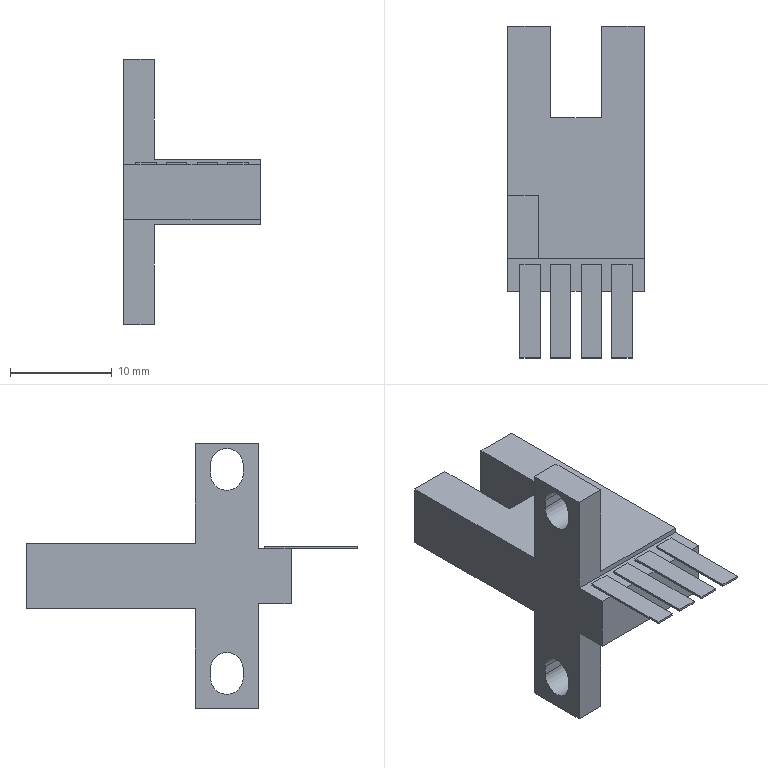Part | SolidWorks | features ICE 6, Extrusion 1, LPattern 1 | 1 solid | 54 faces | box 13.4 x 32.558 x 26 mm | volume 2213 mm3 | plane 48 | cylinder 6 | commonest cylinder face diameters 3.2 x6